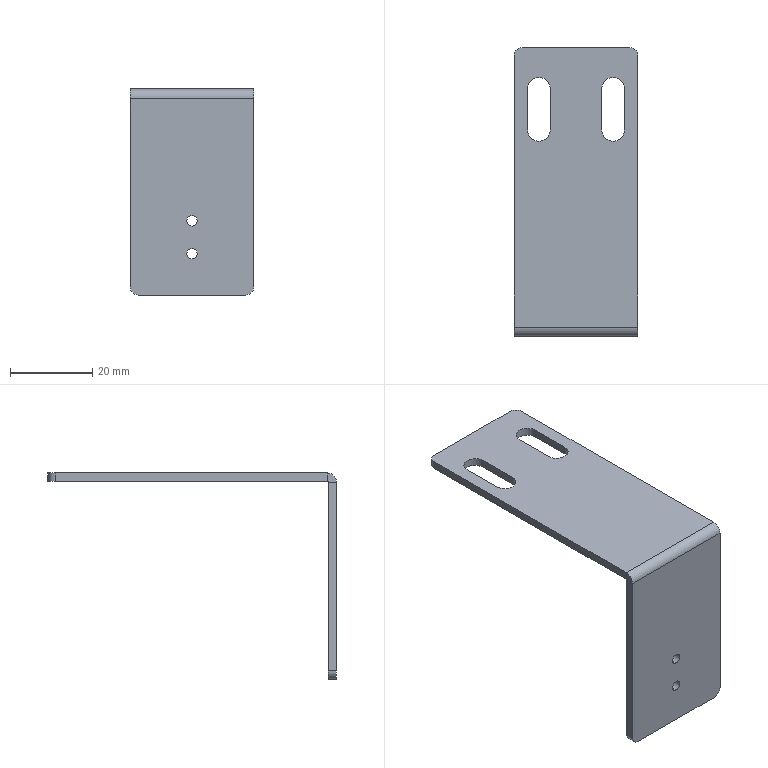Part | STEP file | cable chain mounting plate | 1 solid | 30 faces | box 30 x 70 x 50 mm | volume 6708 mm3 | plane 16 | cylinder 14 | commonest cylinder face diameters 2.5 x4 4 x4 5.5 x4 0.4 x1 4.4 x1